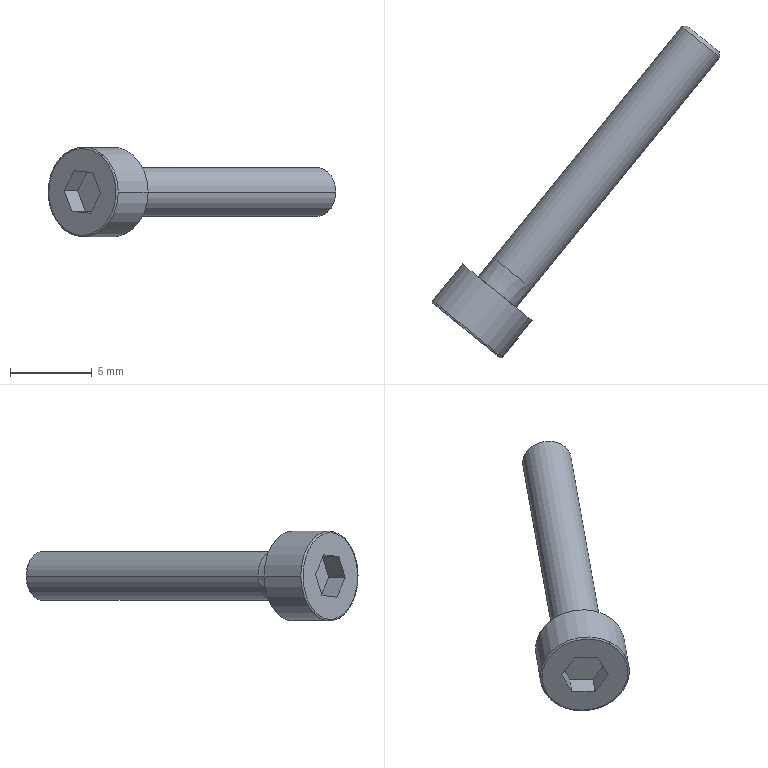Part | SolidWorks | features BaseBody 1 | 1 solid | 20 faces | box 17.61 x 20.327 x 5.5 mm | volume 205.288 mm3 | plane 10 | cylinder 4 | cone 4 | spline 2 | commonest cylinder face diameters 3 x2 5.5 x2
STEP:
#1=CARTESIAN_POINT('',(523.701,-165.581,301.469));
#2=VERTEX_POINT('',#1);
#3=CARTESIAN_POINT('',(524.635,-166.341,299.195));
#4=VERTEX_POINT('',#3);
#5=CARTESIAN_POINT('',(522.501,-164.606,299.195));
#6=DIRECTION('',(0.6309,0.7758,-0.000000012));
#7=DIRECTION('',(-0.7758,0.6309,0.));
#8=AXIS2_PLACEMENT_3D('',#5,#6,#7);
#9=CIRCLE('',#8,2.75);
#10=EDGE_CURVE('',#2,#4,#9,.T.);
#11=ORIENTED_EDGE('',*,*,#10,.F.);
#12=CARTESIAN_POINT('',(523.594,-165.623,301.386));
#13=VERTEX_POINT('',#12);
#14=CARTESIAN_POINT('',(523.657,-165.546,301.386));
#15=DIRECTION('',(0.6417,-0.5218,-0.5621));
#16=DIRECTION('',(0.4361,-0.3546,0.8271));
#17=AXIS2_PLACEMENT_3D('',#14,#15,#16);
#18=CIRCLE('',#17,0.1);
#19=EDGE_CURVE('',#2,#13,#18,.T.);
#20=ORIENTED_EDGE('',*,*,#19,.T.);
#21=CARTESIAN_POINT('',(521.283,-163.744,297.003));
#22=VERTEX_POINT('',#21);
#23=CARTESIAN_POINT('',(523.594,-165.623,301.386));
#24=CARTESIAN_POINT('',(526.995,-168.389,298.407));
#25=CARTESIAN_POINT('',(524.684,-166.51,294.024));
#26=CARTESIAN_POINT('',(521.283,-163.744,297.003));
#27=(BOUNDED_CURVE()B_SPLINE_CURVE(3,(#23,#24,#25,#26),.UNSPECIFIED.,.F.,.F.)B_SPLINE_CURVE_WITH_KNOTS((4,4),(0.,1.),.UNSPECIFIED.)CURVE()GEOMETRIC_REPRESENTATION_ITEM()RATIONAL_B_SPLINE_CURVE((1.,0.3333,0.3333,1.))REPRESENTATION_ITEM(''));
#28=EDGE_CURVE('',#13,#22,#27,.T.);
#29=ORIENTED_EDGE('',*,*,#28,.T.);
#30=CARTESIAN_POINT('',(521.302,-163.631,296.92));
#31=VERTEX_POINT('',#30);
#32=CARTESIAN_POINT('',(521.346,-163.666,297.003));
#33=DIRECTION('',(-0.6417,0.5218,0.5621));
#34=DIRECTION('',(-0.4361,0.3546,-0.8271));
#35=AXIS2_PLACEMENT_3D('',#32,#33,#34);
#36=CIRCLE('',#35,0.1);
#37=EDGE_CURVE('',#31,#22,#36,.T.);
#38=ORIENTED_EDGE('',*,*,#37,.F.);
#39=CARTESIAN_POINT('',(522.501,-164.606,299.195));
#40=DIRECTION('',(0.6309,0.7758,-0.000000012));
#41=DIRECTION('',(-0.7758,0.6309,0.));
#42=AXIS2_PLACEMENT_3D('',#39,#40,#41);
#43=CIRCLE('',#42,2.75);
#44=EDGE_CURVE('',#4,#31,#43,.T.);
#45=ORIENTED_EDGE('',*,*,#44,.F.);
#46=EDGE_LOOP('',(#11,#20,#29,#38,#45));
#47=FACE_OUTER_BOUND('',#46,.T.);
#48=CARTESIAN_POINT('',(523.701,-165.581,301.469));
#49=CARTESIAN_POINT('',(527.23,-168.451,298.378));
#50=CARTESIAN_POINT('',(524.831,-166.501,293.829));
#51=CARTESIAN_POINT('',(521.302,-163.631,296.92));
#52=CARTESIAN_POINT('',(523.664,-165.627,301.469));
#53=CARTESIAN_POINT('',(527.193,-168.497,298.378));
#54=CARTESIAN_POINT('',(524.795,-166.546,293.829));
#55=CARTESIAN_POINT('',(521.265,-163.676,296.92));
#56=CARTESIAN_POINT('',(523.62,-165.644,301.435));
#57=CARTESIAN_POINT('',(527.096,-168.471,298.39));
#58=CARTESIAN_POINT('',(524.733,-166.55,293.909));
#59=CARTESIAN_POINT('',(521.257,-163.723,296.954));
#60=CARTESIAN_POINT('',(523.594,-165.623,301.386));
#61=CARTESIAN_POINT('',(526.995,-168.389,298.407));
#62=CARTESIAN_POINT('',(524.684,-166.51,294.024));
#63=CARTESIAN_POINT('',(521.283,-163.744,297.003));
#64=(BOUNDED_SURFACE()B_SPLINE_SURFACE(3,3,((#48,#49,#50,#51),(#52,#53,#54,#55),(#56,#57,#58,#59),(#60,#61,#62,#63)),.UNSPECIFIED.,.F.,.F.,.T.)B_SPLINE_SURFACE_WITH_KNOTS((4,4),(4,4),(0.,1.),(0.,1.),.UNSPECIFIED.)GEOMETRIC_REPRESENTATION_ITEM()RATIONAL_B_SPLINE_SURFACE(((1.,0.3333,0.3333,1.),(0.8047,0.2682,0.2682,0.8047),(0.8047,0.2682,0.2682,0.8047),(1.,0.3333,0.3333,1.)))REPRESENTATION_ITEM('')SURFACE());
#65=ADVANCED_FACE('',(#47),#64,.T.);
#66=CARTESIAN_POINT('',(524.114,-160.246,299.195));
#67=VERTEX_POINT('',#66);
#68=CARTESIAN_POINT('',(526.441,-162.139,299.195));
#69=VERTEX_POINT('',#68);
#70=CARTESIAN_POINT('',(525.278,-161.192,299.195));
#71=DIRECTION('',(0.6309,0.7758,-0.000000012));
#72=DIRECTION('',(-0.7758,0.6309,0.));
#73=AXIS2_PLACEMENT_3D('',#70,#71,#72);
#74=CIRCLE('',#73,1.5);
#75=EDGE_CURVE('',#67,#69,#74,.T.);
#76=ORIENTED_EDGE('',*,*,#75,.T.);
#77=CARTESIAN_POINT('',(537.956,-147.98,299.195));
#78=VERTEX_POINT('',#77);
#79=CARTESIAN_POINT('',(532.199,-155.059,299.195));
#80=DIRECTION('',(0.6309,0.7758,-0.000000012));
#81=VECTOR('',#80,1000.);
#82=LINE('',#79,#81);
#83=EDGE_CURVE('',#69,#78,#82,.T.);
#84=ORIENTED_EDGE('',*,*,#83,.T.);
#85=CARTESIAN_POINT('',(535.628,-146.087,299.195));
#86=VERTEX_POINT('',#85);
#87=CARTESIAN_POINT('',(536.792,-147.033,299.195));
#88=DIRECTION('',(-0.6309,-0.7758,0.000000012));
#89=DIRECTION('',(-0.7758,0.6309,0.));
#90=AXIS2_PLACEMENT_3D('',#87,#88,#89);
#91=CIRCLE('',#90,1.5);
#92=EDGE_CURVE('',#78,#86,#91,.T.);
#93=ORIENTED_EDGE('',*,*,#92,.T.);
#94=CARTESIAN_POINT('',(529.871,-153.166,299.195));
#95=DIRECTION('',(0.6309,0.7758,-0.000000012));
#96=VECTOR('',#95,1000.);
#97=LINE('',#94,#96);
#98=EDGE_CURVE('',#67,#86,#97,.T.);
#99=ORIENTED_EDGE('',*,*,#98,.F.);
#100=EDGE_LOOP('',(#76,#84,#93,#99));
#101=FACE_OUTER_BOUND('',#100,.T.);
#102=CARTESIAN_POINT('',(531.035,-154.113,299.195));
#103=DIRECTION('',(0.6309,0.7758,-0.000000012));
#104=DIRECTION('',(-0.7758,0.6309,0.));
#105=AXIS2_PLACEMENT_3D('',#102,#103,#104);
#106=CYLINDRICAL_SURFACE('',#105,1.5);
#107=ADVANCED_FACE('',(#101),#106,.T.);
#108=CARTESIAN_POINT('',(523.168,-161.41,299.195));
#109=VERTEX_POINT('',#108);
#110=CARTESIAN_POINT('',(525.494,-163.302,299.195));
#111=VERTEX_POINT('',#110);
#112=CARTESIAN_POINT('',(524.331,-162.356,299.195));
#113=DIRECTION('',(0.6309,0.7758,-0.000000012));
#114=DIRECTION('',(-0.7758,0.6309,0.));
#115=AXIS2_PLACEMENT_3D('',#112,#113,#114);
#116=CIRCLE('',#115,1.499);
#117=EDGE_CURVE('',#109,#111,#116,.T.);
#118=ORIENTED_EDGE('',*,*,#117,.T.);
#119=CARTESIAN_POINT('',(526.441,-162.139,299.195));
#120=DIRECTION('',(0.6313,0.7755,-0.000000012));
#121=VECTOR('',#120,1000.);
#122=LINE('',#119,#121);
#123=EDGE_CURVE('',#111,#69,#122,.T.);
#124=ORIENTED_EDGE('',*,*,#123,.T.);
#125=ORIENTED_EDGE('',*,*,#75,.F.);
#126=CARTESIAN_POINT('',(524.114,-160.246,299.195));
#127=DIRECTION('',(0.6305,0.7762,-0.000000012));
#128=VECTOR('',#127,1000.);
#129=LINE('',#126,#128);
#130=EDGE_CURVE('',#109,#67,#129,.T.);
#131=ORIENTED_EDGE('',*,*,#130,.F.);
#132=EDGE_LOOP('',(#118,#124,#125,#131));
#133=FACE_OUTER_BOUND('',#132,.T.);
#134=CARTESIAN_POINT('',(525.278,-161.192,299.195));
#135=DIRECTION('',(0.6309,0.7758,-0.000000012));
#136=DIRECTION('',(-0.7758,0.6309,0.));
#137=AXIS2_PLACEMENT_3D('',#134,#135,#136);
#138=CONICAL_SURFACE('',#137,1.5,0.0005);
#139=ADVANCED_FACE('',(#133),#138,.T.);
#140=CARTESIAN_POINT('',(537.92,-147.628,299.195));
#141=VERTEX_POINT('',#140);
#142=CARTESIAN_POINT('',(535.98,-146.051,299.195));
#143=VERTEX_POINT('',#142);
#144=CARTESIAN_POINT('',(536.95,-146.839,299.195));
#145=DIRECTION('',(-0.6309,-0.7758,0.000000012));
#146=DIRECTION('',(0.7758,-0.6309,0.));
#147=AXIS2_PLACEMENT_3D('',#144,#145,#146);
#148=CIRCLE('',#147,1.25);
#149=EDGE_CURVE('',#141,#143,#148,.T.);
#150=ORIENTED_EDGE('',*,*,#149,.T.);
#151=CARTESIAN_POINT('',(535.628,-146.087,299.195));
#152=DIRECTION('',(-0.9947,-0.1025,0.000000009));
#153=VECTOR('',#152,1000.);
#154=LINE('',#151,#153);
#155=EDGE_CURVE('',#143,#86,#154,.T.);
#156=ORIENTED_EDGE('',*,*,#155,.T.);
#157=ORIENTED_EDGE('',*,*,#92,.F.);
#158=CARTESIAN_POINT('',(537.956,-147.98,299.195));
#159=DIRECTION('',(0.1025,-0.9947,0.000000009));
#160=VECTOR('',#159,1000.);
#161=LINE('',#158,#160);
#162=EDGE_CURVE('',#141,#78,#161,.T.);
#163=ORIENTED_EDGE('',*,*,#162,.F.);
#164=EDGE_LOOP('',(#150,#156,#157,#163));
#165=FACE_OUTER_BOUND('',#164,.T.);
#166=CARTESIAN_POINT('',(536.792,-147.033,299.195));
#167=DIRECTION('',(-0.6309,-0.7758,0.000000012));
#168=DIRECTION('',(0.7758,-0.6309,0.));
#169=AXIS2_PLACEMENT_3D('',#166,#167,#168);
#170=CONICAL_SURFACE('',#169,1.5,0.7854);
#171=ADVANCED_FACE('',(#165),#170,.T.);
#172=CARTESIAN_POINT('',(520.368,-162.871,299.195));
#173=VERTEX_POINT('',#172);
#174=CARTESIAN_POINT('',(522.501,-164.606,299.195));
#175=DIRECTION('',(0.6309,0.7758,-0.000000012));
#176=DIRECTION('',(-0.7758,0.6309,0.));
#177=AXIS2_PLACEMENT_3D('',#174,#175,#176);
#178=CIRCLE('',#177,2.75);
#179=EDGE_CURVE('',#173,#2,#178,.T.);
#180=ORIENTED_EDGE('',*,*,#179,.T.);
#181=ORIENTED_EDGE('',*,*,#10,.T.);
#182=CARTESIAN_POINT('',(526.465,-164.091,299.195));
#183=VERTEX_POINT('',#182);
#184=CARTESIAN_POINT('',(525.55,-165.216,299.195));
#185=DIRECTION('',(0.6309,0.7758,-0.000000012));
#186=VECTOR('',#185,1000.);
#187=LINE('',#184,#186);
#188=EDGE_CURVE('',#4,#183,#187,.T.);
#189=ORIENTED_EDGE('',*,*,#188,.T.);
#190=CARTESIAN_POINT('',(522.198,-160.621,299.195));
#191=VERTEX_POINT('',#190);
#192=CARTESIAN_POINT('',(524.331,-162.356,299.195));
#193=DIRECTION('',(0.6309,0.7758,-0.000000012));
#194=DIRECTION('',(-0.7758,0.6309,0.));
#195=AXIS2_PLACEMENT_3D('',#192,#193,#194);
#196=CIRCLE('',#195,2.75);
#197=EDGE_CURVE('',#191,#183,#196,.T.);
#198=ORIENTED_EDGE('',*,*,#197,.F.);
#199=CARTESIAN_POINT('',(521.283,-161.746,299.195));
#200=DIRECTION('',(0.6309,0.7758,-0.000000012));
#201=VECTOR('',#200,1000.);
#202=LINE('',#199,#201);
#203=EDGE_CURVE('',#173,#191,#202,.T.);
#204=ORIENTED_EDGE('',*,*,#203,.F.);
#205=EDGE_LOOP('',(#180,#181,#189,#198,#204));
#206=FACE_OUTER_BOUND('',#205,.T.);
#207=CARTESIAN_POINT('',(523.416,-163.481,299.195));
#208=DIRECTION('',(0.6309,0.7758,-0.000000012));
#209=DIRECTION('',(-0.7758,0.6309,0.));
#210=AXIS2_PLACEMENT_3D('',#207,#208,#209);
#211=CYLINDRICAL_SURFACE('',#210,2.75);
#212=ADVANCED_FACE('',(#206),#211,.T.);
#213=ORIENTED_EDGE('',*,*,#83,.F.);
#214=CARTESIAN_POINT('',(525.278,-161.192,299.195));
#215=DIRECTION('',(0.6309,0.7758,-0.000000012));
#216=DIRECTION('',(-0.7758,0.6309,0.));
#217=AXIS2_PLACEMENT_3D('',#214,#215,#216);
#218=CIRCLE('',#217,1.5);
#219=EDGE_CURVE('',#69,#67,#218,.T.);
#220=ORIENTED_EDGE('',*,*,#219,.T.);
#221=ORIENTED_EDGE('',*,*,#98,.T.);
#222=CARTESIAN_POINT('',(536.792,-147.033,299.195));
#223=DIRECTION('',(-0.6309,-0.7758,0.000000012));
#224=DIRECTION('',(-0.7758,0.6309,0.));
#225=AXIS2_PLACEMENT_3D('',#222,#223,#224);
#226=CIRCLE('',#225,1.5);
#227=EDGE_CURVE('',#86,#78,#226,.T.);
#228=ORIENTED_EDGE('',*,*,#227,.T.);
#229=EDGE_LOOP('',(#213,#220,#221,#228));
#230=FACE_OUTER_BOUND('',#229,.T.);
#231=CARTESIAN_POINT('',(531.035,-154.113,299.195));
#232=DIRECTION('',(0.6309,0.7758,-0.000000012));
#233=DIRECTION('',(-0.7758,0.6309,0.));
#234=AXIS2_PLACEMENT_3D('',#231,#232,#233);
#235=CYLINDRICAL_SURFACE('',#234,1.5);
#236=ADVANCED_FACE('',(#230),#235,.T.);
#237=ORIENTED_EDGE('',*,*,#123,.F.);
#238=CARTESIAN_POINT('',(524.331,-162.356,299.195));
#239=DIRECTION('',(0.6309,0.7758,-0.000000012));
#240=DIRECTION('',(-0.7758,0.6309,0.));
#241=AXIS2_PLACEMENT_3D('',#238,#239,#240);
#242=CIRCLE('',#241,1.499);
#243=EDGE_CURVE('',#111,#109,#242,.T.);
#244=ORIENTED_EDGE('',*,*,#243,.T.);
#245=ORIENTED_EDGE('',*,*,#130,.T.);
#246=ORIENTED_EDGE('',*,*,#219,.F.);
#247=EDGE_LOOP('',(#237,#244,#245,#246));
#248=FACE_OUTER_BOUND('',#247,.T.);
#249=CARTESIAN_POINT('',(525.278,-161.192,299.195));
#250=DIRECTION('',(0.6309,0.7758,-0.000000012));
#251=DIRECTION('',(-0.7758,0.6309,0.));
#252=AXIS2_PLACEMENT_3D('',#249,#250,#251);
#253=CONICAL_SURFACE('',#252,1.5,0.0005);
#254=ADVANCED_FACE('',(#248),#253,.T.);
#255=ORIENTED_EDGE('',*,*,#155,.F.);
#256=CARTESIAN_POINT('',(536.95,-146.839,299.195));
#257=DIRECTION('',(-0.6309,-0.7758,0.000000012));
#258=DIRECTION('',(0.7758,-0.6309,0.));
#259=AXIS2_PLACEMENT_3D('',#256,#257,#258);
#260=CIRCLE('',#259,1.25);
#261=EDGE_CURVE('',#143,#141,#260,.T.);
#262=ORIENTED_EDGE('',*,*,#261,.T.);
#263=ORIENTED_EDGE('',*,*,#162,.T.);
#264=ORIENTED_EDGE('',*,*,#227,.F.);
#265=EDGE_LOOP('',(#255,#262,#263,#264));
#266=FACE_OUTER_BOUND('',#265,.T.);
#267=CARTESIAN_POINT('',(536.792,-147.033,299.195));
#268=DIRECTION('',(-0.6309,-0.7758,0.000000012));
#269=DIRECTION('',(0.7758,-0.6309,0.));
#270=AXIS2_PLACEMENT_3D('',#267,#268,#269);
#271=CONICAL_SURFACE('',#270,1.5,0.7854);
#272=ADVANCED_FACE('',(#266),#271,.T.);
#273=ORIENTED_EDGE('',*,*,#117,.F.);
#274=ORIENTED_EDGE('',*,*,#243,.F.);
#275=EDGE_LOOP('',(#273,#274));
#276=FACE_BOUND('',#275,.T.);
#277=ORIENTED_EDGE('',*,*,#197,.T.);
#278=CARTESIAN_POINT('',(524.331,-162.356,299.195));
#279=DIRECTION('',(0.6309,0.7758,-0.000000012));
#280=DIRECTION('',(-0.7758,0.6309,0.));
#281=AXIS2_PLACEMENT_3D('',#278,#279,#280);
#282=CIRCLE('',#281,2.75);
#283=EDGE_CURVE('',#183,#191,#282,.T.);
#284=ORIENTED_EDGE('',*,*,#283,.T.);
#285=EDGE_LOOP('',(#277,#284));
#286=FACE_OUTER_BOUND('',#285,.T.);
#287=CARTESIAN_POINT('',(523.732,-161.869,298.057));
#288=DIRECTION('',(0.6309,0.7758,-0.000000012));
#289=DIRECTION('',(-0.7758,0.6309,0.));
#290=AXIS2_PLACEMENT_3D('',#287,#288,#289);
#291=PLANE('',#290);
#292=ADVANCED_FACE('',(#276,#286),#291,.T.);
#293=ORIENTED_EDGE('',*,*,#149,.F.);
#294=ORIENTED_EDGE('',*,*,#261,.F.);
#295=EDGE_LOOP('',(#293,#294));
#296=FACE_OUTER_BOUND('',#295,.T.);
#297=CARTESIAN_POINT('',(536.677,-146.618,298.678));
#298=DIRECTION('',(0.6309,0.7758,-0.000000012));
#299=DIRECTION('',(-0.7758,0.6309,0.));
#300=AXIS2_PLACEMENT_3D('',#297,#298,#299);
#301=PLANE('',#300);
#302=ADVANCED_FACE('',(#296),#301,.T.);
#303=ORIENTED_EDGE('',*,*,#188,.F.);
#304=ORIENTED_EDGE('',*,*,#44,.T.);
#305=CARTESIAN_POINT('',(522.501,-164.606,299.195));
#306=DIRECTION('',(0.6309,0.7758,-0.000000012));
#307=DIRECTION('',(-0.7758,0.6309,0.));
#308=AXIS2_PLACEMENT_3D('',#305,#306,#307);
#309=CIRCLE('',#308,2.75);
#310=EDGE_CURVE('',#31,#173,#309,.T.);
#311=ORIENTED_EDGE('',*,*,#310,.T.);
#312=ORIENTED_EDGE('',*,*,#203,.T.);
#313=ORIENTED_EDGE('',*,*,#283,.F.);
#314=EDGE_LOOP('',(#303,#304,#311,#312,#313));
#315=FACE_OUTER_BOUND('',#314,.T.);
#316=CARTESIAN_POINT('',(523.416,-163.481,299.195));
#317=DIRECTION('',(0.6309,0.7758,-0.000000012));
#318=DIRECTION('',(-0.7758,0.6309,0.));
#319=AXIS2_PLACEMENT_3D('',#316,#317,#318);
#320=CYLINDRICAL_SURFACE('',#319,2.75);
#321=ADVANCED_FACE('',(#315),#320,.T.);
#322=ORIENTED_EDGE('',*,*,#19,.F.);
#323=ORIENTED_EDGE('',*,*,#179,.F.);
#324=ORIENTED_EDGE('',*,*,#310,.F.);
#325=ORIENTED_EDGE('',*,*,#37,.T.);
#326=CARTESIAN_POINT('',(521.283,-163.744,297.003));
#327=CARTESIAN_POINT('',(517.882,-160.978,299.982));
#328=CARTESIAN_POINT('',(520.193,-162.858,304.365));
#329=CARTESIAN_POINT('',(523.594,-165.623,301.386));
#330=(BOUNDED_CURVE()B_SPLINE_CURVE(3,(#326,#327,#328,#329),.UNSPECIFIED.,.F.,.F.)B_SPLINE_CURVE_WITH_KNOTS((4,4),(0.,1.),.UNSPECIFIED.)CURVE()GEOMETRIC_REPRESENTATION_ITEM()RATIONAL_B_SPLINE_CURVE((1.,0.3333,0.3333,1.))REPRESENTATION_ITEM(''));
#331=EDGE_CURVE('',#22,#13,#330,.T.);
#332=ORIENTED_EDGE('',*,*,#331,.T.);
#333=EDGE_LOOP('',(#322,#323,#324,#325,#332));
#334=FACE_OUTER_BOUND('',#333,.T.);
#335=CARTESIAN_POINT('',(521.302,-163.631,296.92));
#336=CARTESIAN_POINT('',(517.773,-160.761,300.012));
#337=CARTESIAN_POINT('',(520.171,-162.711,304.561));
#338=CARTESIAN_POINT('',(523.701,-165.581,301.469));
#339=CARTESIAN_POINT('',(521.265,-163.676,296.92));
#340=CARTESIAN_POINT('',(517.736,-160.806,300.012));
#341=CARTESIAN_POINT('',(520.134,-162.757,304.561));
#342=CARTESIAN_POINT('',(523.664,-165.627,301.469));
#343=CARTESIAN_POINT('',(521.257,-163.723,296.954));
#344=CARTESIAN_POINT('',(517.781,-160.896,299.999));
#345=CARTESIAN_POINT('',(520.143,-162.817,304.48));
#346=CARTESIAN_POINT('',(523.62,-165.644,301.435));
#347=CARTESIAN_POINT('',(521.283,-163.744,297.003));
#348=CARTESIAN_POINT('',(517.882,-160.978,299.982));
#349=CARTESIAN_POINT('',(520.193,-162.858,304.365));
#350=CARTESIAN_POINT('',(523.594,-165.623,301.386));
#351=(BOUNDED_SURFACE()B_SPLINE_SURFACE(3,3,((#335,#336,#337,#338),(#339,#340,#341,#342),(#343,#344,#345,#346),(#347,#348,#349,#350)),.UNSPECIFIED.,.F.,.F.,.F.)B_SPLINE_SURFACE_WITH_KNOTS((4,4),(4,4),(0.,1.),(0.,1.),.UNSPECIFIED.)GEOMETRIC_REPRESENTATION_ITEM()RATIONAL_B_SPLINE_SURFACE(((1.,0.3333,0.3333,1.),(0.8047,0.2682,0.2682,0.8047),(0.8047,0.2682,0.2682,0.8047),(1.,0.3333,0.3333,1.)))REPRESENTATION_ITEM('')SURFACE());
#352=ADVANCED_FACE('',(#334),#351,.T.);
#353=ORIENTED_EDGE('',*,*,#28,.F.);
#354=ORIENTED_EDGE('',*,*,#331,.F.);
#355=EDGE_LOOP('',(#353,#354));
#356=FACE_OUTER_BOUND('',#355,.T.);
#357=CARTESIAN_POINT('',(521.951,-164.287,300.494));
#358=VERTEX_POINT('',#357);
#359=CARTESIAN_POINT('',(523.068,-165.196,300.388));
#360=VERTEX_POINT('',#359);
#361=CARTESIAN_POINT('',(521.951,-164.287,300.494));
#362=DIRECTION('',(0.7738,-0.6292,-0.07324));
#363=VECTOR('',#362,1000.);
#364=LINE('',#361,#363);
#365=EDGE_CURVE('',#358,#360,#364,.T.);
#366=ORIENTED_EDGE('',*,*,#365,.T.);
#367=CARTESIAN_POINT('',(523.555,-165.592,299.089));
#368=VERTEX_POINT('',#367);
#369=CARTESIAN_POINT('',(523.068,-165.196,300.388));
#370=DIRECTION('',(0.3377,-0.2746,-0.9003));
#371=VECTOR('',#370,1000.);
#372=LINE('',#369,#371);
#373=EDGE_CURVE('',#360,#368,#372,.T.);
#374=ORIENTED_EDGE('',*,*,#373,.T.);
#375=CARTESIAN_POINT('',(522.926,-165.08,297.895));
#376=VERTEX_POINT('',#375);
#377=CARTESIAN_POINT('',(523.555,-165.592,299.089));
#378=DIRECTION('',(-0.4361,0.3546,-0.8271));
#379=VECTOR('',#378,1000.);
#380=LINE('',#377,#379);
#381=EDGE_CURVE('',#368,#376,#380,.T.);
#382=ORIENTED_EDGE('',*,*,#381,.T.);
#383=CARTESIAN_POINT('',(521.809,-164.172,298.001));
#384=VERTEX_POINT('',#383);
#385=CARTESIAN_POINT('',(522.926,-165.08,297.895));
#386=DIRECTION('',(-0.7738,0.6292,0.07324));
#387=VECTOR('',#386,1000.);
#388=LINE('',#385,#387);
#389=EDGE_CURVE('',#376,#384,#388,.T.);
#390=ORIENTED_EDGE('',*,*,#389,.T.);
#391=CARTESIAN_POINT('',(521.322,-163.775,299.3));
#392=VERTEX_POINT('',#391);
#393=CARTESIAN_POINT('',(521.809,-164.172,298.001));
#394=DIRECTION('',(-0.3377,0.2746,0.9003));
#395=VECTOR('',#394,1000.);
#396=LINE('',#393,#395);
#397=EDGE_CURVE('',#384,#392,#396,.T.);
#398=ORIENTED_EDGE('',*,*,#397,.T.);
#399=CARTESIAN_POINT('',(521.322,-163.775,299.3));
#400=DIRECTION('',(0.4361,-0.3546,0.8271));
#401=VECTOR('',#400,1000.);
#402=LINE('',#399,#401);
#403=EDGE_CURVE('',#392,#358,#402,.T.);
#404=ORIENTED_EDGE('',*,*,#403,.T.);
#405=EDGE_LOOP('',(#366,#374,#382,#390,#398,#404));
#406=FACE_BOUND('',#405,.T.);
#407=CARTESIAN_POINT('',(521.861,-164.214,298.099));
#408=DIRECTION('',(-0.6309,-0.7758,0.000000012));
#409=DIRECTION('',(0.7758,-0.6309,0.));
#410=AXIS2_PLACEMENT_3D('',#407,#408,#409);
#411=PLANE('',#410);
#412=ADVANCED_FACE('',(#356,#406),#411,.T.);
#413=CARTESIAN_POINT('',(524.375,-164.583,299.089));
#414=VERTEX_POINT('',#413);
#415=CARTESIAN_POINT('',(523.555,-165.592,299.089));
#416=DIRECTION('',(0.6309,0.7758,0.));
#417=VECTOR('',#416,1000.);
#418=LINE('',#415,#417);
#419=EDGE_CURVE('',#368,#414,#418,.T.);
#420=ORIENTED_EDGE('',*,*,#419,.F.);
#421=ORIENTED_EDGE('',*,*,#373,.F.);
#422=CARTESIAN_POINT('',(523.888,-164.187,300.388));
#423=VERTEX_POINT('',#422);
#424=CARTESIAN_POINT('',(523.068,-165.196,300.388));
#425=DIRECTION('',(-0.6309,-0.7758,0.));
#426=VECTOR('',#425,1000.);
#427=LINE('',#424,#426);
#428=EDGE_CURVE('',#423,#360,#427,.T.);
#429=ORIENTED_EDGE('',*,*,#428,.F.);
#430=CARTESIAN_POINT('',(524.375,-164.583,299.089));
#431=DIRECTION('',(-0.3377,0.2746,0.9003));
#432=VECTOR('',#431,1000.);
#433=LINE('',#430,#432);
#434=EDGE_CURVE('',#414,#423,#433,.T.);
#435=ORIENTED_EDGE('',*,*,#434,.F.);
#436=EDGE_LOOP('',(#420,#421,#429,#435));
#437=FACE_OUTER_BOUND('',#436,.T.);
#438=CARTESIAN_POINT('',(523.555,-165.592,299.089));
#439=DIRECTION('',(0.6985,-0.568,0.4352));
#440=DIRECTION('',(0.6309,0.7758,0.));
#441=AXIS2_PLACEMENT_3D('',#438,#439,#440);
#442=PLANE('',#441);
#443=ADVANCED_FACE('',(#437),#442,.F.);
#444=ORIENTED_EDGE('',*,*,#428,.T.);
#445=ORIENTED_EDGE('',*,*,#365,.F.);
#446=CARTESIAN_POINT('',(522.771,-163.279,300.494));
#447=VERTEX_POINT('',#446);
#448=CARTESIAN_POINT('',(522.771,-163.279,300.494));
#449=DIRECTION('',(-0.6309,-0.7758,0.000000012));
#450=VECTOR('',#449,1000.);
#451=LINE('',#448,#450);
#452=EDGE_CURVE('',#447,#358,#451,.T.);
#453=ORIENTED_EDGE('',*,*,#452,.F.);
#454=CARTESIAN_POINT('',(523.888,-164.187,300.388));
#455=DIRECTION('',(-0.7738,0.6292,0.07324));
#456=VECTOR('',#455,1000.);
#457=LINE('',#454,#456);
#458=EDGE_CURVE('',#423,#447,#457,.T.);
#459=ORIENTED_EDGE('',*,*,#458,.F.);
#460=EDGE_LOOP('',(#444,#445,#453,#459));
#461=FACE_OUTER_BOUND('',#460,.T.);
#462=CARTESIAN_POINT('',(523.068,-165.196,300.388));
#463=DIRECTION('',(0.05682,-0.04621,0.9973));
#464=DIRECTION('',(0.9984,0.,-0.05688));
#465=AXIS2_PLACEMENT_3D('',#462,#463,#464);
#466=PLANE('',#465);
#467=ADVANCED_FACE('',(#461),#466,.F.);
#468=ORIENTED_EDGE('',*,*,#452,.T.);
#469=ORIENTED_EDGE('',*,*,#403,.F.);
#470=CARTESIAN_POINT('',(522.142,-162.767,299.3));
#471=VERTEX_POINT('',#470);
#472=CARTESIAN_POINT('',(522.142,-162.767,299.3));
#473=DIRECTION('',(-0.6309,-0.7758,0.000000012));
#474=VECTOR('',#473,1000.);
#475=LINE('',#472,#474);
#476=EDGE_CURVE('',#471,#392,#475,.T.);
#477=ORIENTED_EDGE('',*,*,#476,.F.);
#478=CARTESIAN_POINT('',(522.771,-163.279,300.494));
#479=DIRECTION('',(-0.4361,0.3546,-0.8271));
#480=VECTOR('',#479,1000.);
#481=LINE('',#478,#480);
#482=EDGE_CURVE('',#447,#471,#481,.T.);
#483=ORIENTED_EDGE('',*,*,#482,.F.);
#484=EDGE_LOOP('',(#468,#469,#477,#483));
#485=FACE_OUTER_BOUND('',#484,.T.);
#486=CARTESIAN_POINT('',(521.951,-164.287,300.494));
#487=DIRECTION('',(-0.6417,0.5218,0.5621));
#488=DIRECTION('',(0.6589,0.,0.7522));
#489=AXIS2_PLACEMENT_3D('',#486,#487,#488);
#490=PLANE('',#489);
#491=ADVANCED_FACE('',(#485),#490,.F.);
#492=ORIENTED_EDGE('',*,*,#476,.T.);
#493=ORIENTED_EDGE('',*,*,#397,.F.);
#494=CARTESIAN_POINT('',(522.629,-163.163,298.001));
#495=VERTEX_POINT('',#494);
#496=CARTESIAN_POINT('',(521.809,-164.172,298.001));
#497=DIRECTION('',(-0.6309,-0.7758,0.));
#498=VECTOR('',#497,1000.);
#499=LINE('',#496,#498);
#500=EDGE_CURVE('',#495,#384,#499,.T.);
#501=ORIENTED_EDGE('',*,*,#500,.F.);
#502=CARTESIAN_POINT('',(522.142,-162.767,299.3));
#503=DIRECTION('',(0.3377,-0.2746,-0.9003));
#504=VECTOR('',#503,1000.);
#505=LINE('',#502,#504);
#506=EDGE_CURVE('',#471,#495,#505,.T.);
#507=ORIENTED_EDGE('',*,*,#506,.F.);
#508=EDGE_LOOP('',(#492,#493,#501,#507));
#509=FACE_OUTER_BOUND('',#508,.T.);
#510=CARTESIAN_POINT('',(521.322,-163.775,299.3));
#511=DIRECTION('',(-0.6985,0.568,-0.4352));
#512=DIRECTION('',(-0.6309,-0.7758,0.));
#513=AXIS2_PLACEMENT_3D('',#510,#511,#512);
#514=PLANE('',#513);
#515=ADVANCED_FACE('',(#509),#514,.F.);
#516=ORIENTED_EDGE('',*,*,#500,.T.);
#517=ORIENTED_EDGE('',*,*,#389,.F.);
#518=CARTESIAN_POINT('',(523.746,-164.071,297.895));
#519=VERTEX_POINT('',#518);
#520=CARTESIAN_POINT('',(523.746,-164.071,297.895));
#521=DIRECTION('',(-0.6309,-0.7758,0.000000012));
#522=VECTOR('',#521,1000.);
#523=LINE('',#520,#522);
#524=EDGE_CURVE('',#519,#376,#523,.T.);
#525=ORIENTED_EDGE('',*,*,#524,.F.);
#526=CARTESIAN_POINT('',(522.629,-163.163,298.001));
#527=DIRECTION('',(0.7738,-0.6292,-0.07324));
#528=VECTOR('',#527,1000.);
#529=LINE('',#526,#528);
#530=EDGE_CURVE('',#495,#519,#529,.T.);
#531=ORIENTED_EDGE('',*,*,#530,.F.);
#532=EDGE_LOOP('',(#516,#517,#525,#531));
#533=FACE_OUTER_BOUND('',#532,.T.);
#534=CARTESIAN_POINT('',(521.809,-164.172,298.001));
#535=DIRECTION('',(-0.05682,0.04621,-0.9973));
#536=DIRECTION('',(-0.9984,0.,0.05688));
#537=AXIS2_PLACEMENT_3D('',#534,#535,#536);
#538=PLANE('',#537);
#539=ADVANCED_FACE('',(#533),#538,.F.);
#540=ORIENTED_EDGE('',*,*,#524,.T.);
#541=ORIENTED_EDGE('',*,*,#381,.F.);
#542=ORIENTED_EDGE('',*,*,#419,.T.);
#543=CARTESIAN_POINT('',(523.746,-164.071,297.895));
#544=DIRECTION('',(0.4361,-0.3546,0.8271));
#545=VECTOR('',#544,1000.);
#546=LINE('',#543,#545);
#547=EDGE_CURVE('',#519,#414,#546,.T.);
#548=ORIENTED_EDGE('',*,*,#547,.F.);
#549=EDGE_LOOP('',(#540,#541,#542,#548));
#550=FACE_OUTER_BOUND('',#549,.T.);
#551=CARTESIAN_POINT('',(522.926,-165.08,297.895));
#552=DIRECTION('',(0.6417,-0.5218,-0.5621));
#553=DIRECTION('',(-0.6589,0.,-0.7522));
#554=AXIS2_PLACEMENT_3D('',#551,#552,#553);
#555=PLANE('',#554);
#556=ADVANCED_FACE('',(#550),#555,.F.);
#557=ORIENTED_EDGE('',*,*,#506,.T.);
#558=ORIENTED_EDGE('',*,*,#530,.T.);
#559=ORIENTED_EDGE('',*,*,#547,.T.);
#560=ORIENTED_EDGE('',*,*,#434,.T.);
#561=ORIENTED_EDGE('',*,*,#458,.T.);
#562=ORIENTED_EDGE('',*,*,#482,.T.);
#563=EDGE_LOOP('',(#557,#558,#559,#560,#561,#562));
#564=FACE_OUTER_BOUND('',#563,.T.);
#565=CARTESIAN_POINT('',(523.259,-163.675,299.195));
#566=DIRECTION('',(-0.6309,-0.7758,0.000000012));
#567=DIRECTION('',(0.7758,-0.6309,0.));
#568=AXIS2_PLACEMENT_3D('',#565,#566,#567);
#569=PLANE('',#568);
#570=ADVANCED_FACE('',(#564),#569,.T.);
#571=CLOSED_SHELL('',(#65,#107,#139,#171,#212,#236,#254,#272,#292,#302,#321,#352,#412,#443,#467,#491,#515,#539,#556,#570));
#572=MANIFOLD_SOLID_BREP('',#571);
#573=CARTESIAN_POINT('',(0.,0.,0.));
#574=DIRECTION('',(0.,0.,1.));
#575=DIRECTION('',(1.,0.,0.));
#576=AXIS2_PLACEMENT_3D('',#573,#574,#575);
#577=(LENGTH_UNIT()NAMED_UNIT(*)SI_UNIT(.MILLI.,.METRE.));
#578=UNCERTAINTY_MEASURE_WITH_UNIT(LENGTH_MEASURE(0.00001),#577,'','');
#579=(NAMED_UNIT(*)PLANE_ANGLE_UNIT()SI_UNIT($,.RADIAN.));
#580=(NAMED_UNIT(*)SI_UNIT($,.STERADIAN.)SOLID_ANGLE_UNIT());
#581=(GEOMETRIC_REPRESENTATION_CONTEXT(3)GLOBAL_UNCERTAINTY_ASSIGNED_CONTEXT((#578))GLOBAL_UNIT_ASSIGNED_CONTEXT((#577,#579,#580))REPRESENTATION_CONTEXT('',''));
#582=ADVANCED_BREP_SHAPE_REPRESENTATION('',(#572,#576),#581);